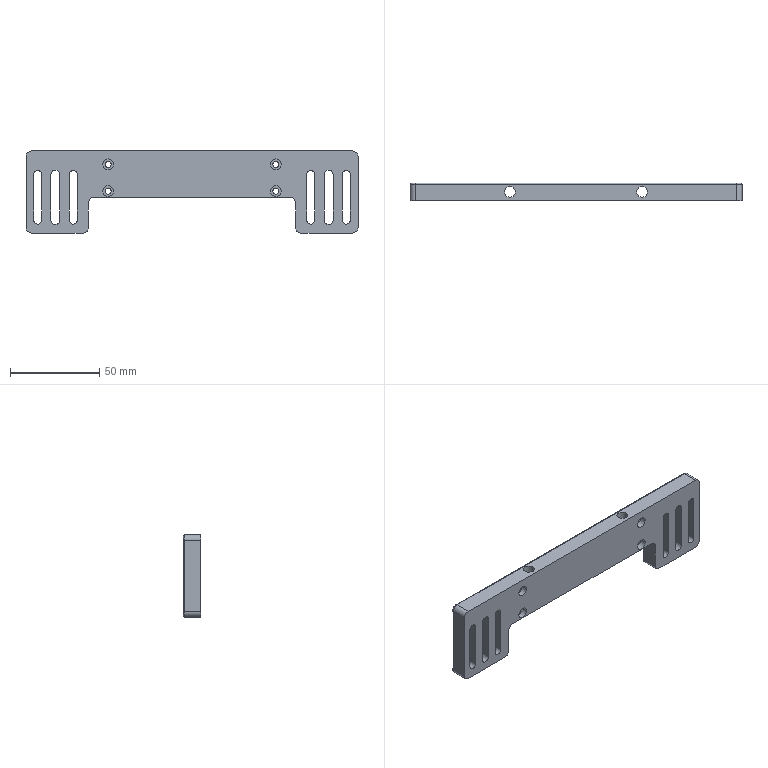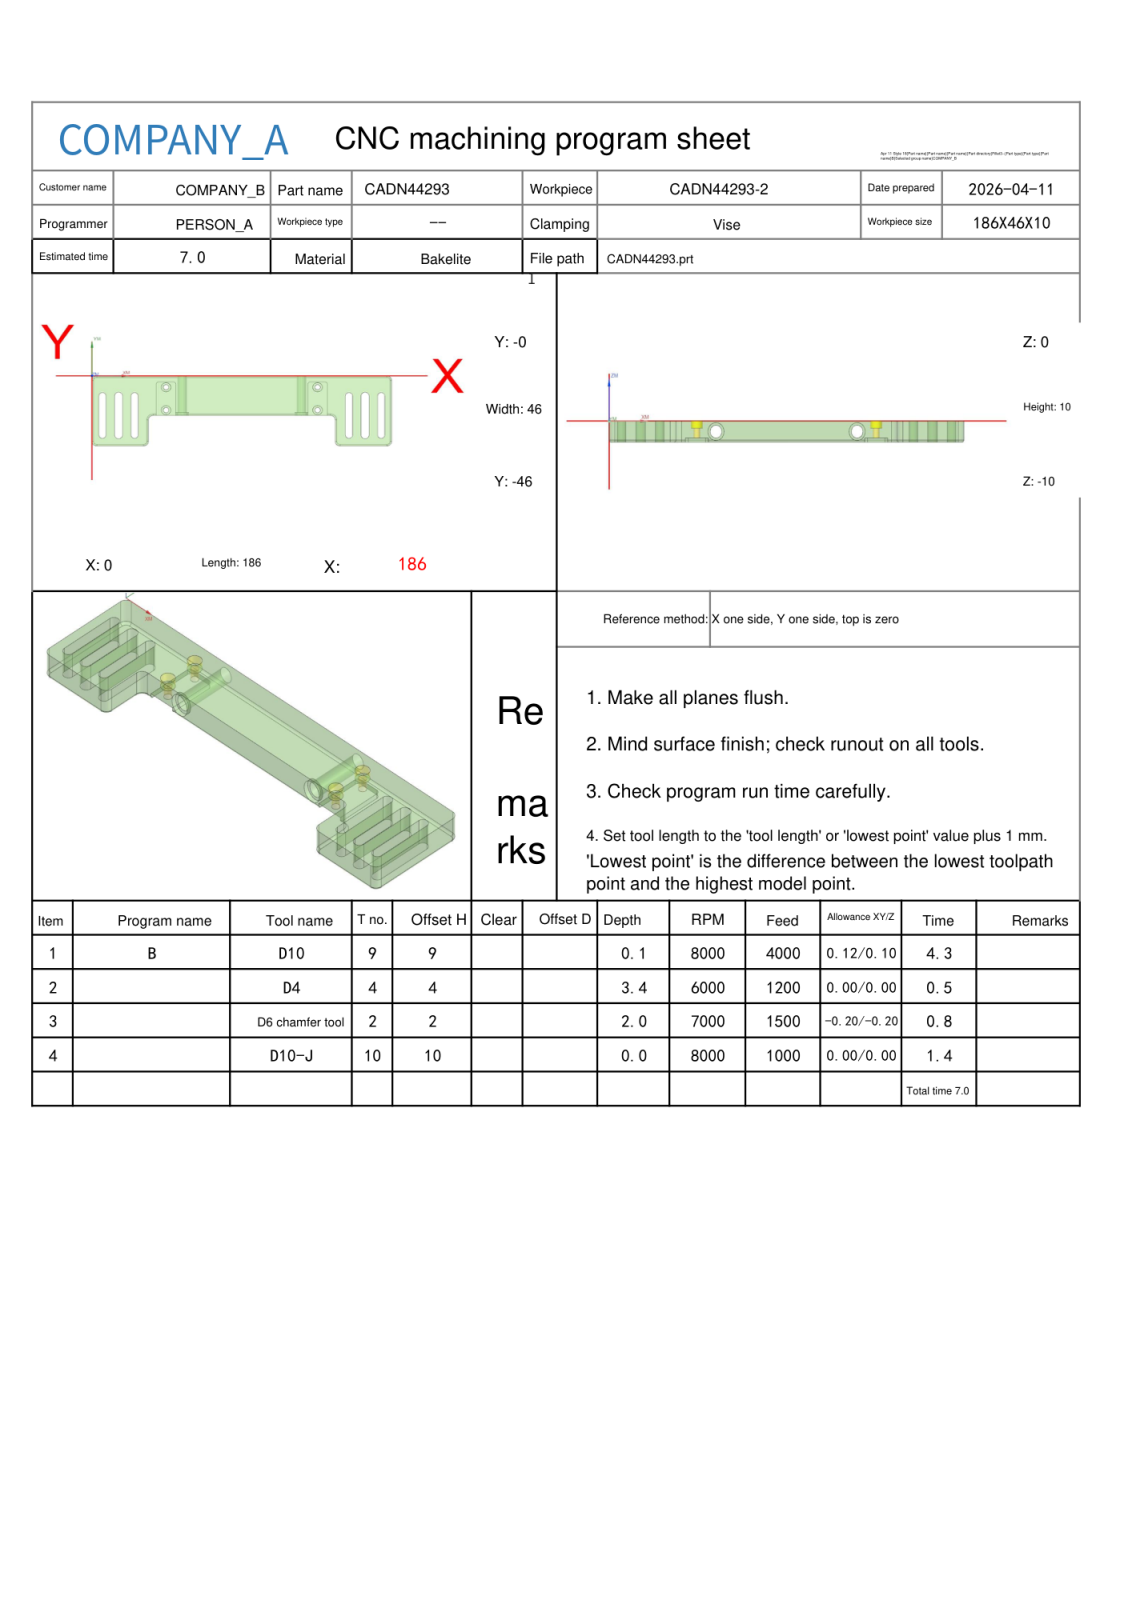NC program | NX | posted by the shop | part box 186 x 10 x 46 mm
Whole program, first 1280 of 1646 lines:
%
O0001
(Machine time: 7.84 MIN)
(===Total Tool:4===)
(T9=D10     D=10.  R=0.   D-  H09 Z=0.1   )
(T4=D4      D=4.   R=0.   D-  H04 Z=-3.4  )
(T2=D6 chamfer tool   D=6.   R=0.   D-  H02 Z=-2.   )
(T10=D10-J  D=10.  R=0.   D-  H10 Z=-0.   )
G80 G90 G17 G49 G40
G91 G28 Z0
M01
N1 T09 M06
(D10  D=10. R=0. H=09 ce=0.12 di=0.10)
G00 G90 G54 X140.535 Y-59.155 M03 S8000
G43 H09 Z20.
M08
Z2.1
G01 X140.517 Y-59.057 Z1.476 F4000.
X140.499 Y-58.958 Z1.228
X140.481 Y-58.86 Z1.046
X140.463 Y-58.762 Z.9
X140.445 Y-58.663 Z.777
X140.427 Y-58.565 Z.672
X140.409 Y-58.466 Z.58
X140.391 Y-58.368 Z.5
X140.373 Y-58.27 Z.43
X140.355 Y-58.171 Z.368
X140.337 Y-58.073 Z.314
X140.319 Y-57.975 Z.267
X140.301 Y-57.876 Z.227
X140.283 Y-57.778 Z.192
X140.265 Y-57.679 Z.164
X140.247 Y-57.581 Z.14
X140.229 Y-57.483 Z.123
X140.211 Y-57.384 Z.11
X140.193 Y-57.286 Z.103
X140.175 Y-57.188 Z.1
X139.761 Y-54.927
G03 X139.47 Y-54.557 I-.503 J-.096
X136.075 Y-54.025 I-3.395 J-10.561
G01 X136.066
G03 X127.645 Y-53.894 I-8.421 J-271.421
X125.75 Y-53.901 I0.0 J-271.551
G01 X-.969 Y-53.881
G02 X-7.111 Y-49.532 I.187 J6.777
X-8.248 Y-43.793 I16.015 J6.156
X-8.42 Y-33.978 I280.233 J9.815
X-8.4 Y-30.595 I280.405 J0.0
G01 X-8.381 Y.463
G02 X-3.982 Y6.632 I6.791 J-.189
X1.641 Y7.744 I6.093 J-16.036
X11.112 Y7.919 I9.47 J-257.315
X14.239 Y7.9 I0.0 J-257.489
G01 X186.963 Y7.881
G02 X193.132 Y3.482 I-.189 J-6.791
X194.244 Y-2.141 I-16.036 J-6.093
X194.419 Y-11.612 I-257.317 J-9.47
X194.4 Y-14.739 I-257.491 J0.0
G01 X194.381 Y-46.463
G02 X189.982 Y-52.632 I-6.791 J.189
X184.359 Y-53.744 I-6.093 J16.036
X174.888 Y-53.919 I-9.47 J257.316
X171.761 Y-53.9 I0.0 J257.49
G01 X141.661 Y-53.882
G03 X128.82 Y-53.296 I-12.842 J-140.443
X127.304 Y-53.304 I0.0 J-141.029
G01 X.611 Y-53.275
G02 X-5.902 Y-48.997 I.391 J7.692
X-7.509 Y-43.008 I14.279 J7.04
X-7.801 Y-35.158 I105.069 J7.85
X-7.793 Y-33.836 I105.362 J0.0
G01 X-7.779 Y-1.213
G02 X-3.481 Y5.41 I7.703 J-.293
X2.636 Y7.023 I7.092 J-14.49
X10.513 Y7.302 I7.877 J-110.962
X11.869 Y7.294 I0.0 J-111.241
G01 X185.288 Y7.279
G02 X191.91 Y2.981 I-.293 J-7.703
X193.523 Y-3.136 I-14.49 J-7.092
X193.803 Y-11.045 I-111.663 J-7.909
X193.794 Y-12.429 I-111.943 J0.0
G01 X193.779 Y-44.787
G02 X189.481 Y-51.41 I-7.703 J.293
X183.364 Y-53.023 I-7.093 J14.49
X175.455 Y-53.303 I-7.909 J111.661
X174.071 Y-53.294 I0.0 J111.941
G01 X143.191 Y-53.284
G03 X133.79 Y-52.797 I-45.842 J-793.897
X123.11 Y-52.701 I-10.916 J-623.13
G01 X2.351 Y-52.681
G02 X-5.271 Y-47.653 I.255 J8.679
X-6.906 Y-41.171 I16.501 J7.608
X-7.206 Y-32.503 I124.946 J8.668
X-7.195 Y-30.798 I125.246 J0.0
G01 X-7.18 Y-2.859
G02 X-2.164 Y4.765 I8.675 J-.246
X4.253 Y6.399 I7.581 J-16.364
X13.347 Y6.713 I9.094 J-131.343
X15.465 Y6.696 I0.0 J-131.658
G01 X183.745 Y6.675
G02 X191.313 Y1.568 I-.354 J-8.685
X192.936 Y-5.164 I-17.162 J-7.7
X193.209 Y-14.034 I-144.224 J-8.87
X193.196 Y-15.958 I-144.497 J0.0
G01 X193.175 Y-43.237
G02 X188.07 Y-50.811 I-8.689 J.349
X181.402 Y-52.431 I-7.671 J17.052
X172.505 Y-52.71 I-8.897 J141.747
X170.548 Y-52.696 I0.0 J142.026
G01 X143.869 Y-52.673
G03 X132.675 Y-52.183 I-42.352 J-839.763
X122.43 Y-52.101 I-10.245 J-640.107
G01 X121.731
X3.851 Y-52.079
G02 X-4.684 Y-46.383 I.148 J9.465
X-6.309 Y-39.529 I18.534 J8.014
X-6.609 Y-30.264 I143.221 J9.265
X-6.595 Y-28.316 I143.521 J0.0
G01 X-6.573 Y-4.277
G02 X-.884 Y4.183 I9.455 J-.216
X5.97 Y5.809 I8.014 J-18.517
X14.918 Y6.104 I8.948 J-135.663
X16.583 Y6.094 I0.0 J-135.958
G01 X182.163 Y6.076
G02 X190.683 Y.385 I-.159 J-9.461
X192.309 Y-6.469 I-18.512 J-8.014
X192.604 Y-15.419 I-135.719 J-8.949
X192.594 Y-17.083 I-136.014 J0.0
G01 X192.576 Y-41.662
G02 X186.885 Y-50.182 I-9.461 J.159
X180.031 Y-51.809 I-8.014 J18.512
X171.084 Y-52.104 I-8.946 J135.482
X169.417 Y-52.094 I0.0 J135.777
G01 X145.138 Y-52.08
G02 X134.437 Y-51.642 I27.7 J808.156
G03 X121.571 Y-51.497 I-12.866 J-571.816
X119.391 Y-51.502 I0.0 J-571.961
G01 X5.351 Y-51.48
X5.261 Y-51.481
G02 X-4.071 Y-45.267 I0.0 J10.116
X-5.708 Y-38.105 I20.101 J8.361
X-6.012 Y-28.177 I161.698 J9.928
X-5.996 Y-25.872 I162.002 J0.0
G01 X-5.975 Y-5.792
Y-5.747
G02 X.174 Y3.544 I10.094 J0.0
X7.328 Y5.202 I8.37 J-19.851
X17.006 Y5.509 I9.677 J-152.413
X19.081 Y5.495 I0.0 J-152.72
G01 X180.701 Y5.476
X180.736
G02 X190.108 Y-.817 I0.0 J-10.126
X191.73 Y-8.166 I-20.695 J-8.421
X192.011 Y-18.022 I-173.11 J-9.857
X191.996 Y-20.28 I-173.39 J0.0
G01 X191.977 Y-40.18
Y-40.235
G02 X185.682 Y-49.609 I-10.127 J0.0
X178.334 Y-51.23 I-8.423 J20.717
X168.479 Y-51.511 I-9.856 J173.021
X166.22 Y-51.496 I0.0 J173.301
G01 X145.9 Y-51.478
G02 X133.852 Y-51.033 I26.655 J884.848
G03 X120.95 Y-50.902 I-13.085 J-653.422
G01 X6.851 Y-50.884
G02 X6.642 Y-50.886 I-.208 J11.472
X.376 Y-49.024 I0.0 J11.474
X-4.028 Y-42.731 I7.031 J9.607
X-5.237 Y-34.805 I29.686 J8.583
X-5.414 Y-23.433 I365.548 J11.372
X-5.398 Y-20.047 I365.725 J0.0
X-5.421 Y-15.221 I506.966 J4.826
X-5.347 Y-6.568 I506.989 J0.0
X1.145 Y2.901 I10.567 J-.285
X8.659 Y4.603 I8.729 J-21.101
X19.063 Y4.914 I10.403 J-173.925
X21.553 Y4.896 I0.0 J-174.235
G01 X179.153 Y4.881
G02 X179.367 Y4.883 I.215 J-11.433
X185.677 Y2.985 I0.0 J-11.435
X190.1 Y-3.497 I-7.196 J-9.659
X191.254 Y-11.554 I-31.403 J-8.608
X191.41 Y-22.82 I-404.751 J-11.265
X191.398 Y-26.013 I-404.907 J0.0
X191.421 Y-30.812 I-504.276 J-4.799
X191.347 Y-39.432 I-504.299 J0.0
X184.855 Y-48.901 I-10.565 J.284
X177.699 Y-50.571 I-8.569 J20.547
X168.131 Y-50.903 I-9.568 J137.881
X166.427 Y-50.892 I0.0 J138.212
G01 X146.167 Y-50.871
G02 X133.382 Y-50.428 I28.171 J997.933
G03 X120.356 Y-50.302 I-13.025 J-673.001
G01 X119.69 Y-50.303
X7.931 Y-50.278
X7.795 Y-50.279
G02 X1.523 Y-48.557 I0.0 J12.286
X-3.319 Y-42.004 I6.721 J10.031
X-4.616 Y-33.91 I29.441 J8.871
X-4.817 Y-22.004 I352.222 J11.906
X-4.798 Y-18.253 I352.423 J0.0
X-4.82 Y-14.666 I288.059 J3.587
X-4.733 Y-7.594 I288.081 J0.0
X2.204 Y2.322 I11.028 J-.33
X9.913 Y4.004 I8.951 J-22.52
X20.05 Y4.307 I10.136 J-169.255
X22.147 Y4.294 I0.0 J-169.558
G01 X177.947 Y4.278
G02 X178.152 Y4.279 I.206 J-12.499
X184.322 Y2.651 I0.0 J-12.501
X189.24 Y-3.769 I-6.443 J-10.029
X190.581 Y-11.491 I-27.39 J-8.736
X190.813 Y-22.407 I-257.318 J-10.917
X190.797 Y-25.287 I-257.549 J0.0
X190.816 Y-29.802 I-531.945 J-4.515
X190.751 Y-38.106 I-531.965 J0.0
X187.925 Y-45.451 I-11.263 J.117
X181.355 Y-49.164 I-9.637 J9.384
X173.212 Y-50.171 I-8.694 J36.869
X161.952 Y-50.305 I-11.26 J473.347
X159.233 Y-50.297 I0.0 J473.481
X154.704 Y-50.32 I-4.529 J444.678
X134.745 Y-49.872 I0.0 J444.702
G03 X119.902 Y-49.698 I-14.843 J-632.459
X117.531 Y-49.703 I0.0 J-632.634
G01 X9.251 Y-49.681
G02 X9.044 Y-49.682 I-.207 J13.728
X3.042 Y-48.301 I0.0 J13.73
X-2.426 Y-41.825 I5.781 J10.428
X-3.939 Y-33.956 I25.86 J9.052
X-4.205 Y-23.7 I197.569 J10.256
X-4.194 Y-21.661 I197.835 J0.0
X-4.221 Y-17.059 I393.597 J4.602
X-4.134 Y-8.782 I393.624 J0.0
X-1.326 Y-1.418 I11.699 J-.244
X5.561 Y2.534 I9.993 J-9.438
X14.42 Y3.585 I9.188 J-39.573
X25.479 Y3.7 I11.059 J-532.946
X27.319 Y3.697 I0.0 J-533.061
G01 X176.879 Y3.672
X177.046 Y3.673
G02 X183.335 Y2.09 I0.0 J-13.281
X188.51 Y-4.4 I-6.313 J-10.343
X189.939 Y-12.044 I-26.458 J-8.899
X190.205 Y-22.403 I-200.887 J-10.359
X190.194 Y-24.519 I-201.154 J0.0
X190.222 Y-29.075 I-377.936 J-4.556
X190.134 Y-37.218 I-377.964 J0.0
X187.326 Y-44.582 I-11.697 J.243
X180.498 Y-48.518 I-9.976 J9.414
X172.119 Y-49.565 I-8.959 J37.652
X157.42 Y-49.721 I-14.7 J691.139
X143.162 Y-49.574 I0.0 J691.296
G03 X120.486 Y-49.093 I-22.676 J-533.468
X117.171 Y-49.103 I0.0 J-533.95
G01 X10.331 Y-49.078
X10.133 Y-49.079
G02 X4.042 Y-47.749 I0.0 J14.611
X-1.72 Y-41.153 I5.623 J10.726
X-3.327 Y-32.997 I26.027 J9.363
X-3.615 Y-21.476 I229.84 J11.521
X-3.596 Y-18.482 I230.129 J0.0
X-3.618 Y-15.7 I173.215 J2.782
X-3.507 Y-9.504 I173.237 J0.0
X-.219 Y-1.715 I11.872 J-.423
X6.809 Y1.999 I10.095 J-10.595
X15.798 Y2.991 I9.314 J-43.16
X27.161 Y3.098 I11.363 J-604.038
X28.637 Y3.096 I0.0 J-604.145
G01 X175.317 Y3.082
G02 X175.659 Y3.085 I.342 J-15.777
X181.42 Y1.996 I0.0 J-15.781
X187.629 Y-4.624 I-4.932 J-10.848
X189.299 Y-12.644 I-24.754 J-9.338
X189.609 Y-23.469 I-189.115 J-10.825
X189.594 Y-25.838 I-189.425 J0.0
X189.619 Y-29.339 I-246.97 J-3.501
X189.52 Y-36.316 I-246.995 J0.0
X186.709 Y-43.758 I-12.125 J.329
X179.772 Y-47.847 I-10.23 J9.425
X171.341 Y-48.949 I-9.14 J37.135
X157.562 Y-49.119 I-13.779 J557.23
X152.523 Y-49.096 I0.0 J557.4
X133.981 Y-48.66 I3.289 J533.594
G03 X118.566 Y-48.499 I-15.415 J-741.74
X116.211 Y-48.503 I0.0 J-741.9
G01 X11.531 Y-48.48
G02 X11.275 Y-48.482 I-.256 J15.943
X5.209 Y-47.283 I0.0 J15.945
X-.983 Y-40.586 I5.226 J11.042
X-2.691 Y-32.394 I25.312 J9.553
X-3.004 Y-21.81 I179.074 J10.585
X-2.992 Y-19.801 I179.386 J0.0
X-3.019 Y-16.815 I167.911 J2.986
X-2.898 Y-10.443 I167.937 J0.0
X.113 Y-2.812 I12.35 J-.463
X7.072 Y1.218 I10.361 J-9.867
X16.04 Y2.359 I9.511 J-38.929
X28.069 Y2.507 I12.029 J-489.04
X31.339 Y2.496 I0.0 J-489.188
G01 X174.298 Y2.478
G02 X174.63 Y2.482 I.332 J-16.513
X180.58 Y1.373 I0.0 J-16.516
X187.005 Y-5.47 I-4.995 J-11.127
X188.695 Y-13.665 I-25.558 J-9.544
X189.001 Y-24.071 I-176.998 J-10.406
X188.991 Y-25.899 I-177.304 J0.0
X189.02 Y-29.043 I-173.951 J-3.145
X188.898 Y-35.557 I-173.979 J0.0
X185.927 Y-43.143 I-12.36 J.465
X178.928 Y-47.218 I-10.386 J9.791
X169.96 Y-48.359 I-9.512 J38.94
X156.764 Y-48.506 I-13.196 J592.148
X133.627 Y-48.054 I0.0 J592.295
G03 X118.417 Y-47.9 I-15.21 J-748.644
X116.031 Y-47.904 I0.0 J-748.798
G01 X12.851 Y-47.885
G02 X12.48 Y-47.889 I-.371 J17.907
X6.49 Y-46.857 I0.0 J17.911
X-.239 Y-40.048 I4.702 J11.375
X-2.027 Y-32.118 I24.119 J9.603
X-2.405 Y-21.19 I157.958 J10.928
X-2.391 Y-19.108 I158.335 J0.0
X-2.419 Y-16.732 I101.932 J2.376
X-2.255 Y-10.951 I101.96 J0.0
X1.678 Y-2.64 I12.276 J-.721
X8.993 Y.867 I10.351 J-12.211
X18.413 Y1.802 I9.658 J-49.349
X29.998 Y1.899 I11.585 J-693.417
X32.032 Y1.896 I0.0 J-693.514
G01 X173.312 Y1.876
G02 X173.619 Y1.878 I.307 J-17.354
X179.662 Y.793 I0.0 J-17.356
X186.337 Y-6.182 I-4.911 J-11.382
X188.044 Y-14.07 I-24.993 J-9.536
X188.406 Y-25.077 I-167.126 J-11.007
X188.391 Y-27.262 I-167.488 J0.0
X188.418 Y-29.492 I-92.94 J-2.23
X188.248 Y-35.117 I-92.967 J0.0
X180.548 Y-45.738 I-12.243 J.774
X172.619 Y-47.526 I-9.601 J24.104
X162.332 Y-47.894 I-10.287 J143.679
X160.868 Y-47.887 I0.0 J144.047
X156.976 Y-47.899 I-3.891 J621.204
X133.451 Y-47.453 I0.0 J621.216
G03 X117.904 Y-47.298 I-15.547 J-776.563
X114.831 Y-47.304 I0.0 J-776.719
G01 X13.871 Y-47.284
G02 X13.504 Y-47.288 I-.367 J19.037
X7.497 Y-46.315 I0.0 J19.04
X.421 Y-39.337 I4.512 J11.651
X-1.429 Y-31.111 I24.615 J9.856
X-1.805 Y-19.964 I165.023 J11.146
X-1.791 Y-17.8 I165.399 J0.0
X-1.815 Y-16.229 I50.679 J1.57
X-1.535 Y-10.91 I50.703 J0.0
X6.162 Y-.922 I12.339 J-1.549
X14.389 Y.929 I9.859 J-24.611
X24.724 Y1.292 I10.335 J-146.724
X26.08 Y1.286 I0.0 J-147.087
G01 X172.28 Y1.275
G02 X172.606 Y1.278 I.326 J-18.32
X178.757 Y.214 I0.0 J-18.323
X185.673 Y-6.885 I-4.83 J-11.625
X187.445 Y-15.069 I-25.449 J-9.792
X187.803 Y-26.05 I-168.253 J-10.981
X187.79 Y-28.081 I-168.611 J0.0
X187.816 Y-29.712 I-51.596 J-1.631
X187.535 Y-35.09 I-51.621 J0.0
X179.838 Y-45.078 I-12.338 J1.549
X171.611 Y-46.928 I-9.857 J24.606
X161.008 Y-47.296 I-10.603 J152.689
X159.38 Y-47.288 I0.0 J153.057
X156.404 Y-47.295 I-2.976 J585.567
X134.284 Y-46.877 I0.0 J585.574
G03 X117.46 Y-46.698 I-16.824 J-789.382
X114.351 Y-46.704 I0.0 J-789.561
G01 X15.131 Y-46.688
G02 X14.673 Y-46.693 I-.458 J21.404
X8.731 Y-45.852 I0.0 J21.409
X1.129 Y-38.752 I4.044 J11.95
X-.787 Y-30.609 I24.062 J9.958
X-1.199 Y-19.568 I147.508 J11.041
X-1.187 Y-17.66 I147.921 J0.0
X-1.207 Y-16.435 I36.406 J1.224
X-.803 Y-11.021 I36.427 J0.0
X6.682 Y-1.66 I12.368 J-2.216
X14.757 Y.273 I9.946 J-23.716
X25.783 Y.698 I11.026 J-142.783
X27.585 Y.687 I0.0 J-143.208
G01 X171.205 Y.675
G02 X171.554 Y.678 I.349 J-19.794
X177.645 Y-.282 I0.0 J-19.798
X184.939 Y-7.401 I-4.467 J-11.871
X186.808 Y-15.615 I-24.76 J-9.954
X187.202 Y-26.648 I-154.165 J-11.033
X187.079 Y-32.823 I-154.559 J0.0
X184.606 Y-40.175 I-13.759 J.537
X177.473 Y-45.056 I-11.129 J8.609
X168.791 Y-46.465 I-9.846 J33.219
X156.255 Y-46.715 I-12.536 J314.508
X151.935 Y-46.685 I0.0 J314.758
X133.216 Y-46.254 I10.619 J867.668
G03 X117.183 Y-46.096 I-16.033 J-812.521
X113.451 Y-46.104 I0.0 J-812.679
G01 X15.611 Y-46.078
G02 X15.32 Y-46.08 I-.291 J20.083
X9.058 Y-45.079 I0.0 J20.085
X1.712 Y-37.902 I4.578 J12.034
X-.208 Y-29.455 I25.178 J10.165
X-.584 Y-19.475 I132.266 J9.981
X-.476 Y-14.107 I132.642 J0.0
X1.837 Y-6.82 I14.277 J-.521
X9.165 Y-1.609 I11.401 J-8.276
X17.959 Y-.147 I10.006 J-33.005
X29.992 Y.109 I12.033 J-281.706
X32.955 Y.094 I0.0 J-281.963
G01 X170.274 Y.073
G02 X170.621 Y.076 I.347 J-20.524
X176.834 Y-.887 I0.0 J-20.527
X184.287 Y-8.098 I-4.453 J-12.059
X186.208 Y-16.544 I-25.199 J-10.172
X186.584 Y-26.531 I-132.468 J-9.987
X186.476 Y-31.892 I-132.844 J0.0
X184.163 Y-39.18 I-14.277 J.521
X176.835 Y-44.391 I-11.4 J8.275
X168.041 Y-45.852 I-10.005 J33.005
X155.322 Y-46.114 I-12.719 J309.509
X149.805 Y-46.065 I0.0 J309.77
X133.514 Y-45.663 I13.249 J869.074
G03 X117.174 Y-45.498 I-16.34 J-804.946
X113.811 Y-45.505 I0.0 J-805.111
G01 X16.691 Y-45.481
G02 X16.343 Y-45.483 I-.348 J21.573
X10.064 Y-44.55 I0.0 J21.576
X2.379 Y-37.257 I4.338 J12.267
X.411 Y-28.76 I25.116 J10.292
X.032 Y-19.77 I106.312 J8.99
X.151 Y-14.733 I106.691 J0.0
X2.695 Y-7.22 I14.222 J-.628
X10.091 Y-2.174 I11.463 J-8.859
X19.132 Y-.733 I10.174 J-34.757
X31.7 Y-.488 I12.569 J-322.02
X35.088 Y-.506 I0.0 J-322.266
G01 X169.168 Y-.524
G02 X169.577 Y-.521 I.409 J-22.208
X175.803 Y-1.411 I0.0 J-22.212
X183.62 Y-8.743 I-4.19 J-12.3
X185.588 Y-17.239 I-25.097 J-10.291
X185.968 Y-26.233 I-106.366 J-8.994
X185.849 Y-31.266 I-106.745 J0.0
X183.3 Y-38.787 I-14.215 J.625
X175.909 Y-43.826 I-11.456 J8.863
X166.868 Y-45.267 I-10.173 J34.76
X154.123 Y-45.508 I-12.745 J335.947
X143.533 Y-45.341 I0.0 J336.189
G03 X116.656 Y-44.895 I-26.877 J-809.372
X112.731 Y-44.905 I0.0 J-809.818
G01 X17.651 Y-44.881
G02 X17.312 Y-44.884 I-.339 J22.944
X11.072 Y-44.019 I0.0 J22.946
X3.012 Y-36.548 I4.095 J12.5
X1.058 Y-28.351 I24.804 J10.245
X.652 Y-20.109 I83.523 J8.242
X.798 Y-15.167 I83.928 J0.0
X3.834 Y-7.278 I13.891 J-.817
X11.245 Y-2.665 I11.387 J-10.034
X20.186 Y-1.326 I10.139 J-37.173
X33.776 Y-1.084 I13.59 J-381.581
X37.883 Y-1.106 I0.0 J-381.823
G01 X168.543 Y-1.131
G02 X168.861 Y-1.129 I.319 J-21.557
X175.34 Y-2.126 I0.0 J-21.559
X183.029 Y-9.547 I-4.542 J-12.399
X184.964 Y-17.875 I-25.349 J-10.279
X185.345 Y-25.96 I-85.61 J-8.085
X185.214 Y-30.7 I-85.991 J0.0
X182.437 Y-38.387 I-14.115 J.755
X175.041 Y-43.246 I-11.479 J9.414
X166.053 Y-44.661 I-10.207 J35.586
X153.626 Y-44.901 I-12.428 J321.198
X142.718 Y-44.716 I0.0 J321.438
G03 X116.2 Y-44.295 I-26.518 J-835.167
X112.131 Y-44.305 I0.0 J-835.588
G01 X18.851 Y-44.286
G02 X18.384 Y-44.29 I-.467 J25.098
X12.08 Y-43.486 I0.0 J25.102
X3.664 Y-35.892 I3.836 J12.713
X1.674 Y-27.642 I24.841 J10.357
X1.287 Y-20.24 I70.738 J7.402
X1.416 Y-15.958 I71.124 J0.0
X4.446 Y-7.997 I14.09 J-.806
X11.959 Y-3.29 I11.533 J-10.061
X21.255 Y-1.916 I10.374 J-38.054
X34.724 Y-1.685 I13.469 J-392.231
X38.772 Y-1.706 I0.0 J-392.462
G01 X167.212 Y-1.724
G02 X167.679 Y-1.72 I.467 J-24.604
X174.038 Y-2.555 I0.0 J-24.609
X182.335 Y-10.107 I-3.95 J-12.673
X184.326 Y-18.357 I-24.822 J-10.356
X184.712 Y-25.764 I-70.75 J-7.407
X184.584 Y-30.041 I-71.137 J0.0
X181.563 Y-37.991 I-14.087 J.803
X174.041 Y-42.709 I-11.532 J10.03
X164.745 Y-44.083 I-10.374 J38.055
X153.135 Y-44.286 I-11.61 J331.976
X141.23 Y-44.073 I0.0 J332.179
G03 X116.13 Y-43.697 I-25.1 J-838.204
X112.431 Y-43.705 I0.0 J-838.58
G01 X19.511 Y-43.681
G02 X19.129 Y-43.684 I-.382 J24.834
X12.686 Y-42.834 I0.0 J24.837
X4.238 Y-35.075 I4.015 J12.851
X2.264 Y-26.696 I25.626 J10.46
X1.924 Y-20.554 I55.352 J6.142
X2.093 Y-16.213 I55.692 J0.0
X6.418 Y-7.289 I13.544 J-1.054
X13.948 Y-3.563 I11.163 J-13.085
X23.648 Y-2.45 I10.418 J-47.982
X36.744 Y-2.296 I13.096 J-556.098
X40.207 Y-2.306 I0.0 J-556.252
G01 X166.547 Y-2.329
G02 X166.939 Y-2.326 I.392 J-24.3
X173.426 Y-3.207 I0.0 J-24.304
X181.722 Y-10.839 I-4.109 J-12.792
X183.756 Y-19.505 I-25.694 J-10.601
X184.077 Y-25.432 I-54.56 J-5.927
X183.898 Y-29.868 I-54.881 J0.0
X179.372 Y-38.895 I-13.462 J1.101
X171.735 Y-42.513 I-11.138 J13.644
X161.667 Y-43.573 I-10.549 J51.816
X153.215 Y-43.652 I-8.452 J451.504
X136.621 Y-43.347 I0.0 J451.583
G03 X115.685 Y-43.095 I-20.936 J-869.43
X111.471 Y-43.106 I0.0 J-869.682
G01 X20.711 Y-43.087
G02 X20.192 Y-43.092 I-.519 J27.197
X13.695 Y-42.304 I0.0 J27.202
X4.915 Y-34.499 I3.728 J13.034
X2.855 Y-25.774 I25.803 J10.699
X2.571 Y-20.796 I43.483 J4.978
X2.789 Y-16.432 I43.767 J0.0
X11.139 Y-5.359 I13.476 J-1.477
X19.515 Y-3.377 I10.513 J-25.73
X30.661 Y-2.918 I11.146 J-135.126
X31.862 Y-2.923 I0.0 J-135.585
G01 X165.642 Y-2.929
G02 X166.033 Y-2.926 I.392 J-25.486
X172.529 Y-3.767 I0.0 J-25.489
X181.083 Y-11.5 I-3.948 J-12.965
X183.138 Y-20.167 I-25.703 J-10.674
X183.429 Y-25.204 I-43.584 J-5.037
X183.211 Y-29.568 I-43.874 J0.0
X174.861 Y-40.641 I-13.474 J1.476
X166.127 Y-42.659 I-10.678 J26.307
X154.557 Y-43.086 I-11.569 J156.511
X151.318 Y-43.052 I0.0 J156.938
X132.507 Y-42.653 I11.255 J972.573
G03 X115.927 Y-42.494 I-16.58 J-867.96
X111.471 Y-42.506 I0.0 J-868.118
G01 X21.671 Y-42.488
G02 X21.117 Y-42.493 I-.554 J28.694
X14.589 Y-41.741 I0.0 J28.699
X5.49 Y-33.7 I3.594 J13.236
X3.471 Y-25.084 I26.065 J10.652
X3.23 Y-21.015 I34.29 J4.069
X3.523 Y-16.526 I34.53 J0.0
X11.584 Y-6.094 I13.383 J-2.01
X19.938 Y-4.018 I10.62 J-24.895
X31.359 Y-3.518 I11.422 J-130.002
X32.643 Y-3.524 I0.0 J-130.502
G01 X164.743 Y-3.529
G02 X165.163 Y-3.526 I.421 J-26.344
X171.753 Y-4.363 I0.0 J-26.347
X180.469 Y-12.212 I-3.912 J-13.109
X182.536 Y-20.995 I-25.939 J-10.739
X182.771 Y-24.989 I-33.916 J-3.994
X182.464 Y-29.552 I-34.15 J0.0
X174.415 Y-39.907 I-13.364 J2.082
X165.704 Y-42.019 I-10.778 J25.431
X154.413 Y-42.475 I-11.292 J139.582
X151.677 Y-42.448 I0.0 J140.038
X132.269 Y-42.05 I10.342 J976.217
G03 X115.772 Y-41.894 I-16.497 J-875.327
X111.231 Y-41.906 I0.0 J-875.483
G01 X22.031 Y-41.88
G02 X21.648 Y-41.882 I-.383 J26.761
X14.963 Y-41.034 I0.0 J26.764
X6.128 Y-33.054 I3.947 J13.251
X4.069 Y-24.148 I26.072 J10.718
X3.901 Y-21.162 I26.352 J2.986
X4.357 Y-16.263 I26.521 J0.0
X12.212 Y-6.745 I13.227 J-2.915
X20.916 Y-4.6 I10.851 J-25.304
X32.293 Y-4.119 I11.377 J-134.401
X33.502 Y-4.125 I0.0 J-134.881
G01 X163.922 Y-4.13
G02 X164.323 Y-4.127 I.401 J-27.186
X170.934 Y-4.943 I0.0 J-27.189
X179.905 Y-13.026 I-3.852 J-13.295
X181.957 Y-22.176 I-26.602 J-10.773
X182.102 Y-24.888 I-25.375 J-2.712
X181.597 Y-29.937 I-25.519 J0.0
X173.787 Y-39.255 I-13.179 J3.113
X165.084 Y-41.4 I-10.84 J25.261
X153.742 Y-41.869 I-11.343 J136.996
X150.698 Y-41.835 I0.0 J137.465
X132.27 Y-41.452 I11.38 J990.771
G03 X115.675 Y-41.295 I-16.595 J-878.031
X111.171 Y-41.307 I0.0 J-878.188
G01 X23.171 Y-41.285
G02 X22.688 Y-41.289 I-.483 J29.422
X16.03 Y-40.526 I0.0 J29.426
X6.729 Y-32.329 I3.613 J13.475
X4.638 Y-22.34 I26.311 J10.722
X4.589 Y-20.998 I18.451 J1.342
X5.664 Y-14.784 I18.5 J0.0
X13.108 Y-7.27 I12.739 J-5.177
X21.764 Y-5.195 I10.826 J-26.06
X33.531 Y-4.713 I11.767 J-143.57
X35.071 Y-4.721 I0.0 J-144.052
G01 X162.791 Y-4.726
G02 X163.328 Y-4.721 I.537 J-29.259
X170.049 Y-5.503 I0.0 J-29.264
X179.206 Y-13.531 I-3.661 J-13.412
X181.349 Y-23.386 I-25.855 J-10.782
X181.412 Y-24.937 I-18.883 J-1.551
X180.392 Y-31.071 I-18.946 J0.0
X172.892 Y-38.73 I-12.782 J5.016
X164.235 Y-40.805 I-10.821 J26.045
X153.05 Y-41.259 I-11.185 J137.466
X149.728 Y-41.219 I0.0 J137.92
X133.404 Y-40.876 I9.946 J862.354
G03 X115.469 Y-40.695 I-17.935 J-888.588
X110.931 Y-40.707 I0.0 J-888.768
G01 X24.071 Y-40.686
G02 X23.572 Y-40.69 I-.499 J30.913
X16.924 Y-39.967 I0.0 J30.917
X7.379 Y-31.721 I3.43 J13.618
X5.34 Y-21.694 I23.641 J10.027
X5.571 Y-18.263 I25.68 J0.0
X13.304 Y-8.119 I13.318 J-2.133
X21.734 Y-5.886 I10.878 J-24.029
X33.42 Y-5.323 I11.686 J-121.196
X34.616 Y-5.329 I0.0 J-121.758
G01 X161.915 Y-5.326
G02 X162.432 Y-5.321 I.516 J-31.053
X169.063 Y-6.038 I0.0 J-31.057
X178.618 Y-14.278 I-3.408 J-13.612
X180.659 Y-24.31 I-23.636 J-10.032
X180.43 Y-27.736 I-25.677 J0.0
X172.696 Y-37.881 I-13.317 J2.131
X164.266 Y-40.114 I-10.869 J24.007
X153.198 Y-40.645 I-11.068 J114.992
X150.783 Y-40.62 I0.0 J115.523
X133.226 Y-40.274 I8.686 J887.192
G03 X115.397 Y-40.096 I-17.829 J-891.639
X110.871 Y-40.107 I0.0 J-891.817
G01 X24.911 Y-40.086
G02 X24.364 Y-40.091 I-.546 J31.269
X17.527 Y-39.335 I0.0 J31.274
X7.981 Y-31.01 I3.543 J13.699
X6.084 Y-21.871 I21.071 J9.139
X6.291 Y-18.794 I22.968 J0.0
X13.915 Y-8.775 I13.227 J-2.156
X22.347 Y-6.505 I10.933 J-23.816
X33.888 Y-5.931 I11.541 J-115.573
X34.808 Y-5.934 I0.0 J-116.148
G01 X161.088 Y-5.926
G02 X161.645 Y-5.921 I.557 J-31.409
X168.414 Y-6.659 I0.0 J-31.413
X178.054 Y-15.074 I-3.49 J-13.728
X179.916 Y-24.092 I-20.902 J-9.018
X179.673 Y-27.412 I-22.764 J0.0
X172.098 Y-37.218 I-13.189 J2.359
X163.736 Y-39.483 I-10.891 J23.636
X152.883 Y-40.03 I-10.853 J107.326
X150.795 Y-40.01 I0.0 J107.874
X131.795 Y-39.648 I9.417 J992.722
G03 X115.328 Y-39.496 I-16.467 J-891.378
X110.751 Y-39.508 I0.0 J-891.53
G01 X25.631 Y-39.485
G02 X25.111 Y-39.489 I-.52 J31.545
X18.247 Y-38.733 I0.0 J31.549
X8.57 Y-30.271 I3.528 J13.799
X6.851 Y-22.107 I18.529 J8.164
X7.1 Y-18.941 I20.247 J0.0
X14.419 Y-9.487 I13.018 J-2.518
X23.057 Y-7.113 I11.098 J-23.478
X34.408 Y-6.538 I11.351 J-111.801
X35.037 Y-6.54 I0.0 J-112.376
G01 X46.257 Y-6.509
X160.597 Y-6.531
G02 X161.05 Y-6.528 I.453 J-30.186
X167.916 Y-7.319 I0.0 J-30.189
X177.402 Y-15.67 I-3.671 J-13.733
X179.149 Y-23.895 I-18.488 J-8.225
X178.9 Y-27.056 I-20.235 J0.0
X171.581 Y-36.513 I-13.02 J2.516
X162.99 Y-38.879 I-11.052 J23.352
X152.099 Y-39.422 I-10.892 J108.973
X149.629 Y-39.394 I0.0 J109.516
X132.989 Y-39.072 I8.814 J885.768
G03 X115.181 Y-38.896 I-17.809 J-901.818
X110.571 Y-38.908 I0.0 J-901.994
G01 X26.771 Y-38.89
G02 X26.171 Y-38.895 I-.6 J35.222
X19.374 Y-38.233 I0.0 J35.227
X9.152 Y-29.509 I3.102 J13.986
X7.645 Y-22.303 I16.471 J7.206
X7.909 Y-19.23 I17.978 J0.0
X15.034 Y-10.145 I12.832 J-2.726
X23.302 Y-7.779 I10.976 J-22.731
X35.067 Y-7.136 I11.765 J-107.268
X35.938 Y-7.139 I0.0 J-107.911
G01 X47.158 Y-7.109
X159.758 Y-7.131
G02 X160.244 Y-7.127 I.486 J-30.918
X167.198 Y-7.919 I0.0 J-30.922
X176.844 Y-16.489 I-3.654 J-13.827
X178.354 Y-23.678 I-16.36 J-7.189
X178.053 Y-26.943 I-17.87 J0.0
X170.966 Y-35.855 I-12.797 J2.903
X162.459 Y-38.248 I-11.043 J22.94
X151.726 Y-38.807 I-10.733 J102.832
X149.519 Y-38.783 I0.0 J103.391
X132.811 Y-38.47 I7.626 J852.133
G03 X115.038 Y-38.296 I-17.773 J-908.959
X110.331 Y-38.308 I0.0 J-909.133
G01 X27.071 Y-38.283
G02 X26.596 Y-38.286 I-.475 J32.064
X19.628 Y-37.52 I0.0 J32.067
X9.654 Y-28.522 I3.522 J13.931
X8.467 Y-22.549 I14.426 J5.973
X8.905 Y-18.873 I15.614 J0.0
X15.756 Y-10.751 I12.506 J-3.597
X24.381 Y-8.338 I11.127 J-23.154
X36.014 Y-7.737 I11.633 J-112.29
X36.78 Y-7.739 I0.0 J-112.891
G01 X48.179 Y-7.71
X158.919 Y-7.731
G02 X159.419 Y-7.727 I.5 J-32.082
X166.363 Y-8.488 I0.0 J-32.086
X176.337 Y-17.461 I-3.503 J-13.922
X177.532 Y-23.452 I-14.411 J-5.99
X177.097 Y-27.111 I-15.607 J0.0
X170.243 Y-35.249 I-12.509 J3.579
X161.975 Y-37.611 I-10.934 J22.629
X151.225 Y-38.194 I-10.75 J98.744
X149.037 Y-38.17 I0.0 J99.327
X131.559 Y-37.849 I9.291 J980.679
G03 X114.532 Y-37.693 I-17.027 J-934.01
X109.191 Y-37.709 I0.0 J-934.166
G01 X27.911 Y-37.684
G02 X27.428 Y-37.687 I-.483 J33.36
X20.463 Y-36.952 I0.0 J33.364
X10.001 Y-26.965 I3.352 J13.985
X9.31 Y-22.756 I12.475 J4.209
X10.539 Y-17.201 I13.166 J0.0
X17.367 Y-10.931 I12.047 J-6.266
X25.962 Y-8.842 I10.937 J-26.28
X37.645 Y-8.328 I11.683 J-132.443
X38.667 Y-8.332 I0.0 J-132.958
G01 X157.807 Y-8.327
G02 X158.418 Y-8.321 I.611 J-35.063
X165.379 Y-9.019 I0.0 J-35.068
X175.995 Y-19.03 I-3.193 J-14.02
X176.688 Y-23.242 I-12.455 J-4.212
X175.407 Y-28.902 I-13.148 J0.0
X168.63 Y-35.069 I-12.008 J6.388
X159.854 Y-37.167 I-10.932 J26.335
X149.533 Y-37.583 I-10.321 J127.812
X145.886 Y-37.531 I0.0 J128.228
G01 X126.546 Y-37.179
X109.431 Y-37.109
X28.771 Y-37.085
G02 X28.259 Y-37.089 I-.512 J34.697
X21.26 Y-36.376 I0.0 J34.7
X10.241 Y-22.704 I2.972 J13.672
X10.308 Y-21.338 I13.991 J0.0
X16.3 Y-12.483 I11.986 J-1.656
X24.27 Y-9.773 I11.028 J-19.36
X35.618 Y-8.977 I11.349 J-80.449
G01 X35.632
G02 X46.166 Y-8.902 I10.534 J-745.037
X49.612 Y-8.91 I0.0 J-745.112
G01 X157.052 Y-8.927
G02 X157.636 Y-8.923 I.584 J-36.058
X164.568 Y-9.595 I0.0 J-36.062
X175.755 Y-23.287 I-2.784 J-13.692
X175.677 Y-24.769 I-13.972 J0.0
X169.686 Y-33.525 I-11.976 J1.767
X161.527 Y-36.251 I-11.052 J19.498
X150.968 Y-36.954 I-10.559 J79.036
X149.739 Y-36.944 I0.0 J79.738
X131.56 Y-36.651 I5.242 J890.284
G03 X114.388 Y-36.495 I-17.172 J-939.638
X109.131 Y-36.509 I0.0 J-939.795
G01 X29.491 Y-36.484
G02 X28.983 Y-36.488 I-.508 J34.908
X21.92 Y-35.766 I0.0 J34.911
X11.316 Y-24.822 I2.847 J13.368
X11.18 Y-23.071 I11.187 J1.751
X16.071 Y-13.752 I11.323 J0.0
X23.918 Y-10.576 I11.151 J-16.267
X34.422 Y-9.623 I11.051 J-63.417
X47.542 Y-9.506 I13.12 J-735.95
X50.262 Y-9.511 I0.0 J-736.067
G01 X156.561 Y-9.532
G02 X157.058 Y-9.528 I.497 J-34.741
X164.072 Y-10.243 I0.0 J-34.744
X174.678 Y-21.156 I-2.833 J-13.363
X174.818 Y-22.932 I-11.179 J-1.775
X169.929 Y-32.247 I-11.319 J0.0
X162.196 Y-35.393 I-11.056 J16.099
X151.672 Y-36.309 I-10.524 J59.984
G01 X151.449
X150.566
G02 X131.202 Y-36.047 I0.0 J714.692
G03 X114.174 Y-35.894 I-17.029 J-949.403
X108.771 Y-35.91 I0.0 J-949.555
G01 X30.631 Y-35.89
G02 X30.018 Y-35.895 I-.613 J38.749
X22.991 Y-35.252 I0.0 J38.754
X13.71 Y-28.783 I2.539 J13.535
X12.187 Y-23.26 I9.252 J5.523
X16.518 Y-14.624 I10.776 J0.0
X23.985 Y-11.325 I10.997 J-14.791
X34.475 Y-10.245 I11.122 J-56.558
X47.984 Y-10.104 I13.509 J-648.212
X50.973 Y-10.111 I0.0 J-648.352
G01 X156.073 Y-10.136
G02 X156.491 Y-10.134 I.418 J-33.46
X163.579 Y-10.893 I0.0 J-33.462
X172.935 Y-18.525 I-2.903 J-13.11
X173.806 Y-22.761 I-9.864 J-4.236
X169.504 Y-31.356 I-10.735 J0.0
X161.921 Y-34.686 I-10.993 J14.736
X151.353 Y-35.686 I-10.567 J55.306
G01 X151.244
G02 X148.336 Y-35.694 I-2.907 J564.984
X132.338 Y-35.467 I0.0 J564.991
G03 X114.083 Y-35.294 I-18.255 J-962.603
X108.591 Y-35.31 I0.0 J-962.776
G01 X31.411 Y-35.29
G02 X30.764 Y-35.295 I-.647 J39.227
X23.651 Y-34.645 I0.0 J39.232
X15.263 Y-29.451 I2.515 J13.433
X13.251 Y-23.396 I8.109 J6.055
X16.826 Y-15.678 I10.12 J0.0
X23.983 Y-12.114 I10.873 J-12.867
X33.372 Y-10.92 I10.664 J-46.339
X47.995 Y-10.691 I14.623 J-465.973
X52.389 Y-10.711 I0.0 J-466.202
G01 X155.329 Y-10.737
G02 X155.779 Y-10.734 I.449 J-33.516
X163.011 Y-11.524 I0.0 J-33.519
X171.292 Y-17.405 I-2.926 J-12.89
X172.744 Y-22.619 I-8.632 J-5.214
X169.201 Y-30.294 I-10.084 J0.0
X161.967 Y-33.887 I-10.862 J12.791
X152.091 Y-35.033 I-10.367 J46.212
X145.995 Y-35.083 I-6.096 J372.055
X134.67 Y-34.91 I0.0 J372.105
G03 X114.003 Y-34.694 I-20.668 J-984.645
X108.291 Y-34.71 I0.0 J-984.862
G01 X32.191 Y-34.69
G02 X31.506 Y-34.696 I-.685 J39.671
X24.312 Y-34.039 I0.0 J39.677
X16.627 Y-29.646 I2.476 J13.252
X14.378 Y-23.525 I7.207 J6.122
X17.246 Y-16.741 I9.456 J0.0
X24.253 Y-12.861 I10.76 J-11.161
X33.502 Y-11.553 I10.621 J-41.782
X46.495 Y-11.302 I12.992 J-335.443
X49.279 Y-11.314 I0.0 J-335.695
G01 X154.559 Y-11.337
G02 X155.004 Y-11.334 I.445 J-34.519
X162.186 Y-12.089 I0.0 J-34.522
X169.79 Y-16.903 I-2.743 J-12.743
X171.618 Y-22.484 I-7.604 J-5.58
X168.765 Y-29.242 I-9.432 J0.0
X161.922 Y-33.076 I-10.647 J10.978
X152.493 Y-34.377 I-10.281 J39.694
X145.415 Y-34.481 I-7.077 J239.276
X138.635 Y-34.385 I0.0 J239.381
G03 X115.798 Y-34.108 I-22.837 J-939.366
X112.547 Y-34.113 I0.0 J-939.643
G01 X32.911 Y-34.09
G02 X32.221 Y-34.096 I-.69 J39.927
X24.971 Y-33.433 I0.0 J39.933
X17.976 Y-29.7 I2.416 J12.951
X15.579 Y-23.655 I6.424 J6.045
X17.907 Y-17.683 I8.822 J0.0
X24.592 Y-13.612 I10.507 J-9.73
X33.521 Y-12.199 I10.468 J-37.218
X46.723 Y-11.899 I13.203 J-290.777
X49.656 Y-11.914 I0.0 J-291.077
G01 X153.856 Y-11.938
G02 X154.299 Y-11.935 I.444 J-34.681
X161.541 Y-12.7 I0.0 J-34.684
X168.453 Y-16.81 I-2.647 J-12.319
X170.416 Y-22.351 I-6.843 J-5.541
X168.086 Y-28.317 I-8.805 J0.0
X161.458 Y-32.355 I-10.432 J9.667
X152.225 Y-33.74 I-10.18 J36.384
X144.794 Y-33.869 I-7.431 J214.055
X138.848 Y-33.787 I0.0 J214.184
G03 X115.676 Y-33.507 I-23.172 J-959.09
X112.127 Y-33.513 I0.0 J-959.37
G01 X33.271 Y-33.485
G02 X32.712 Y-33.489 I-.559 J37.837
X25.457 Y-32.787 I0.0 J37.841
X19.074 Y-29.392 I2.355 J12.123
X16.866 Y-23.787 I6.012 J5.605
X18.734 Y-18.57 I8.22 J0.0
X24.892 Y-14.413 I10.114 J-8.342
X33.607 Y-12.849 I10.317 J-32.433
X45.656 Y-12.513 I12.049 J-215.568
X47.461 Y-12.52 I0.0 J-215.905
G01 X153.101 Y-12.538
G02 X153.552 Y-12.535 I.452 J-35.371
X160.789 Y-13.283 I0.0 J-35.374
X166.968 Y-16.667 I-2.494 J-11.889
X169.127 Y-22.214 I-6.048 J-5.547
X167.243 Y-27.446 I-8.207 J0.0
X160.956 Y-31.619 I-10.102 J8.398
X152.041 Y-33.095 I-9.999 J32.726
X143.878 Y-33.257 I-8.163 J205.229
X137.704 Y-33.164 I0.0 J205.392
G03 X115.021 Y-32.902 I-22.683 J-980.712
X110.509 Y-32.912 I0.0 J-980.974
G01 X34.051 Y-32.886
G02 X33.458 Y-32.891 I-.593 J38.444
X26.176 Y-32.195 I0.0 J38.449
X20.471 Y-29.307 I2.163 J11.353
X18.257 Y-23.926 I5.432 J5.381
X19.708 Y-19.443 I7.646 J0.0
X25.594 Y-15.114 I9.777 J-7.126
X34.051 Y-13.48 I10.087 J-29.511
X46.197 Y-13.111 I12.146 J-199.828
X48.143 Y-13.121 I0.0 J-200.196
G01 X152.043 Y-13.133
G02 X152.593 Y-13.13 I.55 J-38.406
X159.741 Y-13.8 I0.0 J-38.409
X165.512 Y-16.69 I-2.113 J-11.431
X167.734 Y-22.074 I-5.415 J-5.384
X166.25 Y-26.597 I-7.637 J0.0
X160.407 Y-30.86 I-9.695 J7.155
X152.001 Y-32.431 I-9.704 J28.639
X143.616 Y-32.647 I-8.385 J162.576
X139.046 Y-32.583 I0.0 J162.792
G03 X115.852 Y-32.31 I-23.194 J-986.077
X112.726 Y-32.315 I0.0 J-986.35
G01 X34.831 Y-32.287
G02 X34.238 Y-32.291 I-.593 J39.699
X27.071 Y-31.639 I0.0 J39.704
X21.893 Y-29.134 I1.835 J10.398
X19.775 Y-24.066 I5.004 J5.068
X20.92 Y-20.195 I7.122 J0.0
X26.472 Y-15.789 I9.377 J-6.117
X34.376 Y-14.129 I9.668 J-26.38
X45.777 Y-13.724 I11.401 J-160.117
X47.026 Y-13.728 I0.0 J-160.522
G01 X151.646 Y-13.739
G02 X152.119 Y-13.736 I.473 J-35.94
X159.277 Y-14.456 I0.0 J-35.943
X164.4 Y-17.185 I-1.903 J-9.743
X166.21 Y-21.931 I-5.317 J-4.746
X165.028 Y-25.863 I-7.127 J0.0
X159.427 Y-30.215 I-9.325 J6.219
X151.329 Y-31.802 I-9.395 J26.495
X142.563 Y-32.033 I-8.765 J165.673
X137.474 Y-31.955 I0.0 J165.905
G03 X115.639 Y-31.71 I-21.835 J-970.483
X112.306 Y-31.715 I0.0 J-970.729
G01 X35.551 Y-31.687
G02 X34.952 Y-31.691 I-.599 J39.956
X27.909 Y-31.065 I0.0 J39.96
X23.291 Y-28.795 I1.49 J8.86
X21.451 Y-24.199 I4.818 J4.596
X22.413 Y-20.75 I6.659 J0.0
X27.767 Y-16.349 I8.993 J-5.484
X35.309 Y-14.733 I9.258 J-24.786
X46.771 Y-14.32 I11.462 J-158.913
X48.259 Y-14.327 I0.0 J-159.326
G01 X150.539 Y-14.333
G02 X151.084 Y-14.33 I.545 J-40.149
X158.004 Y-14.931 I0.0 J-40.153
X162.694 Y-17.209 I-1.436 J-8.921
X164.53 Y-21.796 I-4.813 J-4.587
X163.529 Y-25.304 I-6.648 J0.0
X158.201 Y-29.617 I-8.913 J5.564
X150.463 Y-31.179 I-9.005 J24.655
X141.988 Y-31.417 I-8.475 J151.
X137.628 Y-31.354 I0.0 J151.237
G03 X115.931 Y-31.114 I-21.697 J-979.516
X113.204 Y-31.118 I0.0 J-979.757
G01 X36.211 Y-31.086
G02 X35.64 Y-31.09 I-.571 J39.78
X28.865 Y-30.509 I0.0 J39.784
X24.534 Y-28.037 I1.102 J6.962
X23.333 Y-24.315 I5.165 J3.721
X24.38 Y-20.817 I6.366 J0.0
X29.57 Y-16.767 I8.607 J-5.679
X37.078 Y-15.271 I8.956 J-25.357
X48.975 Y-14.908 I11.897 J-194.636
X51.17 Y-14.92 I0.0 J-194.999
G01 X149.79 Y-14.933
G02 X150.415 Y-14.928 I.625 J-39.144
X157.195 Y-15.52 I0.0 J-39.149
X161.568 Y-18.136 I-1.095 J-6.793
X162.636 Y-21.665 I-5.297 J-3.529
X161.558 Y-25.21 I-6.365 J0.0
X156.244 Y-29.237 I-8.553 J5.765
X148.714 Y-30.611 I-8.556 J25.576
X140.792 Y-30.794 I-7.923 J171.636
X135.998 Y-30.727 I0.0 J171.819
G03 X115.664 Y-30.513 I-20.334 J-964.85
X112.665 Y-30.517 I0.0 J-965.064
G01 X36.931 Y-30.486
G02 X36.335 Y-30.491 I-.596 J38.969
X30.059 Y-29.982 I0.0 J38.974
X25.446 Y-24.488 I.965 J5.494
X25.819 Y-22.482 I5.578 J0.0
X30.24 Y-17.78 I8.004 J-3.096
X37.113 Y-15.986 I8.466 J-18.376
X47.847 Y-15.524 I10.733 J-124.255
X49.22 Y-15.531 I0.0 J-124.718
G01 X149.1 Y-15.534
G02 X149.66 Y-15.53 I.561 J-39.658
X155.854 Y-16.017 I0.0 J-39.662
X160.503 Y-21.484 I-.89 J-5.467
X160.154 Y-23.417 I-5.539 J0.0
X155.755 Y-28.134 I-7.917 J2.973
X149.108 Y-29.852 I-8.073 J17.519
X141.026 Y-30.183 I-8.082 J98.53
X138.558 Y-30.152 I0.0 J98.861
G01 X118.712 Y-29.937
X37.291 Y-29.881
G02 X36.758 Y-29.885 I-.532 J33.214
X31.731 Y-29.503 I0.0 J33.219
X27.95 Y-24.673 I1.195 J4.83
X28.064 Y-23.613 I4.975 J0.0
X31.806 Y-18.611 I7.364 J-1.607
X37.887 Y-16.686 I7.835 J-14.183
X47.252 Y-16.15 I9.365 J-81.572
X47.826 Y-16.152 I0.0 J-82.107
G01 X59.226 Y-16.115
X148.366 Y-16.134
G02 X148.917 Y-16.13 I.551 J-38.4
X154.109 Y-16.483 I0.0 J-38.404
X157.958 Y-21.283 I-1.07 J-4.8
X157.85 Y-22.306 I-4.918 J0.0
X154.151 Y-27.28 I-7.273 J1.547
X147.813 Y-29.194 I-7.712 J14.082
X140.024 Y-29.563 I-7.789 J82.206
X137.925 Y-29.536 I0.0 J82.575
G01 X118.293 Y-29.336
X38.071 Y-29.282
G02 X37.515 Y-29.288 I-.556 J25.095
X34.301 Y-29.082 I0.0 J25.101
X31.04 Y-24.86 I1.102 J4.221
X31.052 Y-24.541 I4.363 J0.0
X34.053 Y-19.427 I6.66 J-.471
X39.75 Y-17.319 I7.399 J-11.244
X48.315 Y-16.754 I8.565 J-64.69
X48.845 Y-16.757 I0.0 J-65.254
G01 X60.664 Y-16.715
X147.584 Y-16.734
G02 X148.054 Y-16.73 I.47 J-33.71
X151.477 Y-16.905 I0.0 J-33.713
X154.772 Y-21.05 I-.96 J-4.145
G01 X154.769 Y-21.213
G02 X151.943 Y-26.341 I-6.486 J.232
X146.319 Y-28.468 I-7.189 J10.509
X139.11 Y-28.93 I-7.21 J55.997
X137.82 Y-28.915 I0.0 J56.459
G01 X117.395 Y-28.733
X39.091 Y-28.686
G02 X38.723 Y-28.704 I-.368 J3.656
X36.55 Y-27.993 I0.0 J3.675
X35.045 Y-24.597 I3.079 J3.396
X35.553 Y-22.499 I4.584 J0.0
X39.998 Y-18.673 I7.01 J-3.65
X46.287 Y-17.514 I6.949 J-20.071
X55.903 Y-17.307 I9.615 J-222.862
X58.044 Y-17.317 I0.0 J-223.07
G01 X147.364 Y-17.342
G02 X150.13 Y-19.345 I-.228 J-3.227
X150.564 Y-21.409 I-4.699 J-2.064
X148.734 Y-25.337 I-5.133 J0.0
X143.341 Y-27.791 I-6.923 J8.064
X136.55 Y-28.294 I-6.791 J45.594
X135.326 Y-28.277 I0.0 J46.097
G01 X113.023 Y-28.121
X43.052 Y-28.094
G02 X40.498 Y-25.017 I1.278 J3.658
X40.428 Y-24.148 I5.315 J.869
X44.596 Y-18.901 I5.386 J0.0
X51.24 Y-18.02 I6.829 J-26.001
X61.558 Y-17.91 I10.318 J-484.083
X63.839 Y-17.916 I0.0 J-484.193
G01 X142.32 Y-17.94
G02 X144.918 Y-21.79 I-1.554 J-3.85
G01 X144.917 Y-21.903
G02 X141.505 Y-26.91 I-5.488 J.074
X134.934 Y-27.625 I-6.571 J29.842
X134.477 Y-27.622 I0.0 J30.557
X131.273 Y-27.627 I-3.205 J891.486
X119.069 Y-27.544 I0.0 J891.492
G01 X53.931 Y-27.513
G02 X49.875 Y-27.925 I-5.811 J37.018
G01 X49.776 Y-27.934 Z.103
X49.676 Y-27.942 Z.11
X49.576 Y-27.951 Z.123
X49.477 Y-27.96 Z.14
X49.377 Y-27.968 Z.164
X49.278 Y-27.977 Z.192
X49.178 Y-27.986 Z.227
X49.078 Y-27.994 Z.267
X48.979 Y-28.003 Z.314
X48.879 Y-28.011 Z.368
X48.779 Y-28.02 Z.43
X48.68 Y-28.029 Z.5
X48.58 Y-28.037 Z.58
X48.481 Y-28.046 Z.672
X48.381 Y-28.054 Z.777
X48.281 Y-28.063 Z.9
X48.182 Y-28.072 Z1.046
X48.082 Y-28.08 Z1.228
X47.982 Y-28.089 Z1.476
X47.883 Y-28.097 Z2.1
G00 Z20.
G91 G28 Z0.0
M05
M09
G91 G28 Z0.0
M01
N2 T04 M06
(D4  D=4. R=0. H=04 ce=0.07 di=0.00)
G00 G90 G54 X46. Y-22.5 M03 S6000
G43 H04 Z20.
M08
Z.3
G03 X46.465 Y-22.965 I.465 J0.0 F1200.
X46.93 Y-22.5 I0.0 J.465
X46.93 Y-22.5 Z.1 I-.93 J0.0
X46.93 Y-22.5 Z-.1 I-.93 J0.0
X46.93 Y-22.5 Z-.3 I-.93 J0.0
X46.93 Y-22.5 Z-.5 I-.93 J0.0
X46.93 Y-22.5 Z-.7 I-.93 J0.0
X46.93 Y-22.5 Z-.9 I-.93 J0.0
X46.93 Y-22.5 Z-1.1 I-.93 J0.0
X46.93 Y-22.5 Z-1.3 I-.93 J0.0
X46.93 Y-22.5 Z-1.5 I-.93 J0.0
X46.93 Y-22.5 Z-1.7 I-.93 J0.0
X46.93 Y-22.5 Z-1.9 I-.93 J0.0
X46.93 Y-22.5 Z-2.1 I-.93 J0.0
X46.93 Y-22.5 Z-2.3 I-.93 J0.0
X46.93 Y-22.5 Z-2.5 I-.93 J0.0
X46.93 Y-22.5 Z-2.7 I-.93 J0.0
X46.93 Y-22.5 Z-2.9 I-.93 J0.0
X46.93 Y-22.5 Z-3.1 I-.93 J0.0
X46.93 Y-22.5 Z-3.3 I-.93 J0.0
X45.07 Y-22.5 Z-3.4 I-.93 J0.0
X46. Y-23.43 I.93 J0.0
X46.93 Y-22.5 I0.0 J.93
X46. Y-21.57 I-.93 J0.0
X45.07 Y-22.5 I0.0 J-.93
X45.535 Y-22.965 I.465 J0.0
X46. Y-22.5 I0.0 J.465
G00 Z20.
Y-7.5
Z.3
G03 X46.465 Y-7.965 I.465 J0.0
X46.93 Y-7.5 I0.0 J.465
X46.93 Y-7.5 Z.1 I-.93 J0.0
X46.93 Y-7.5 Z-.1 I-.93 J0.0
X46.93 Y-7.5 Z-.3 I-.93 J0.0
X46.93 Y-7.5 Z-.5 I-.93 J0.0
X46.93 Y-7.5 Z-.7 I-.93 J0.0
X46.93 Y-7.5 Z-.9 I-.93 J0.0
X46.93 Y-7.5 Z-1.1 I-.93 J0.0
X46.93 Y-7.5 Z-1.3 I-.93 J0.0
X46.93 Y-7.5 Z-1.5 I-.93 J0.0
X46.93 Y-7.5 Z-1.7 I-.93 J0.0
X46.93 Y-7.5 Z-1.9 I-.93 J0.0
X46.93 Y-7.5 Z-2.1 I-.93 J0.0
X46.93 Y-7.5 Z-2.3 I-.93 J0.0
X46.93 Y-7.5 Z-2.5 I-.93 J0.0
X46.93 Y-7.5 Z-2.7 I-.93 J0.0
X46.93 Y-7.5 Z-2.9 I-.93 J0.0
X46.93 Y-7.5 Z-3.1 I-.93 J0.0
X46.93 Y-7.5 Z-3.3 I-.93 J0.0
X45.07 Y-7.5 Z-3.4 I-.93 J0.0
X46. Y-8.43 I.93 J0.0
X46.93 Y-7.5 I0.0 J.93
X46. Y-6.57 I-.93 J0.0
X45.07 Y-7.5 I0.0 J-.93
X45.535 Y-7.965 I.465 J0.0
X46. Y-7.5 I0.0 J.465
G00 Z20.
X140.
Z.3
G03 X140.465 Y-7.965 I.465 J0.0
X140.93 Y-7.5 I0.0 J.465
X140.93 Y-7.5 Z.1 I-.93 J0.0
X140.93 Y-7.5 Z-.1 I-.93 J0.0
X140.93 Y-7.5 Z-.3 I-.93 J0.0
X140.93 Y-7.5 Z-.5 I-.93 J0.0
X140.93 Y-7.5 Z-.7 I-.93 J0.0
X140.93 Y-7.5 Z-.9 I-.93 J0.0
X140.93 Y-7.5 Z-1.1 I-.93 J0.0
X140.93 Y-7.5 Z-1.3 I-.93 J0.0
X140.93 Y-7.5 Z-1.5 I-.93 J0.0
X140.93 Y-7.5 Z-1.7 I-.93 J0.0
X140.93 Y-7.5 Z-1.9 I-.93 J0.0
X140.93 Y-7.5 Z-2.1 I-.93 J0.0
X140.93 Y-7.5 Z-2.3 I-.93 J0.0
X140.93 Y-7.5 Z-2.5 I-.93 J0.0
X140.93 Y-7.5 Z-2.7 I-.93 J0.0
X140.93 Y-7.5 Z-2.9 I-.93 J0.0
X140.93 Y-7.5 Z-3.1 I-.93 J0.0
X140.93 Y-7.5 Z-3.3 I-.93 J0.0
X139.07 Y-7.5 Z-3.4 I-.93 J0.0
X140. Y-8.43 I.93 J0.0
X140.93 Y-7.5 I0.0 J.93
X140. Y-6.57 I-.93 J0.0
X139.07 Y-7.5 I0.0 J-.93
X139.535 Y-7.965 I.465 J0.0
X140. Y-7.5 I0.0 J.465
G00 Z20.
Y-22.5
Z.3
G03 X140.465 Y-22.965 I.465 J0.0
X140.93 Y-22.5 I0.0 J.465
X140.93 Y-22.5 Z.1 I-.93 J0.0
X140.93 Y-22.5 Z-.1 I-.93 J0.0
X140.93 Y-22.5 Z-.3 I-.93 J0.0
X140.93 Y-22.5 Z-.5 I-.93 J0.0
X140.93 Y-22.5 Z-.7 I-.93 J0.0
X140.93 Y-22.5 Z-.9 I-.93 J0.0
X140.93 Y-22.5 Z-1.1 I-.93 J0.0
X140.93 Y-22.5 Z-1.3 I-.93 J0.0
X140.93 Y-22.5 Z-1.5 I-.93 J0.0
X140.93 Y-22.5 Z-1.7 I-.93 J0.0
X140.93 Y-22.5 Z-1.9 I-.93 J0.0
X140.93 Y-22.5 Z-2.1 I-.93 J0.0
X140.93 Y-22.5 Z-2.3 I-.93 J0.0
X140.93 Y-22.5 Z-2.5 I-.93 J0.0
X140.93 Y-22.5 Z-2.7 I-.93 J0.0
X140.93 Y-22.5 Z-2.9 I-.93 J0.0
X140.93 Y-22.5 Z-3.1 I-.93 J0.0
X140.93 Y-22.5 Z-3.3 I-.93 J0.0
X139.07 Y-22.5 Z-3.4 I-.93 J0.0
X140. Y-23.43 I.93 J0.0
X140.93 Y-22.5 I0.0 J.93
X140. Y-21.57 I-.93 J0.0
X139.07 Y-22.5 I0.0 J-.93
X139.535 Y-22.965 I.465 J0.0
X140. Y-22.5 I0.0 J.465
G00 Z20.
G00 G90 X46. Y-22.5 M03 S6000
Z20.
Z-3.4
G01 X46.568 Y-22.772 F600.
X46.698 Y-22.802
G03 X47. Y-22.5 I0.0 J.302
X46. Y-21.5 I-1. J0.0
X45. Y-22.5 I0.0 J-1.
X46. Y-23.5 I1. J0.0
X47. Y-22.5 I0.0 J1.
X46.878 Y-22.021 I-1. J0.0
X46.613 Y-21.864 I-.265 J-.145
X46.368 Y-21.989 I0.0 J-.302
G01 X46. Y-22.5
G00 Z20.
Y-7.5